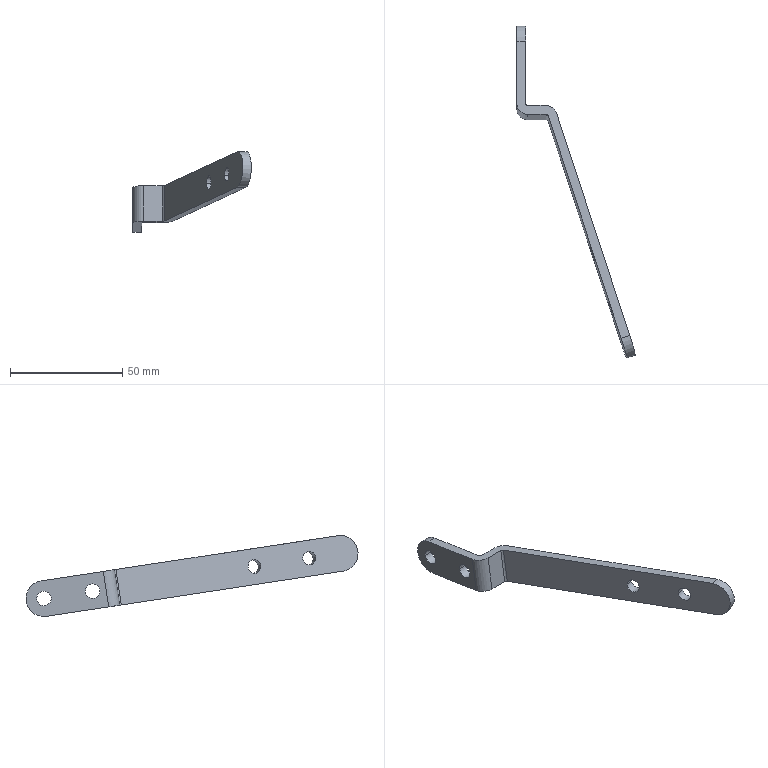Part | SolidWorks | features BaseBody 1 | 1 solid | 23 faces | box 52.887 x 148.089 x 36.172 mm | volume 9906 mm3 | cylinder 15 | plane 8 | commonest cylinder face diameters 6.1 x4 6.5 x4 16 x3 2 x2 10 x2
STEP:
#1=CARTESIAN_POINT('',(27.037,49.349,-203.779));
#2=VERTEX_POINT('',#1);
#3=CARTESIAN_POINT('',(27.037,42.645,-194.665));
#4=VERTEX_POINT('',#3);
#5=CARTESIAN_POINT('',(27.037,41.44,-202.574));
#6=DIRECTION('',(1.,0.,0.));
#7=DIRECTION('',(0.,0.9886,-0.1506));
#8=AXIS2_PLACEMENT_3D('',#5,#6,#7);
#9=CIRCLE('',#8,8.);
#10=EDGE_CURVE('',#2,#4,#9,.T.);
#11=ORIENTED_EDGE('',*,*,#10,.F.);
#12=CARTESIAN_POINT('',(23.037,49.349,-203.779));
#13=VERTEX_POINT('',#12);
#14=CARTESIAN_POINT('',(23.037,49.349,-203.779));
#15=DIRECTION('',(-1.,0.,0.));
#16=VECTOR('',#15,1000.);
#17=LINE('',#14,#16);
#18=EDGE_CURVE('',#2,#13,#17,.T.);
#19=ORIENTED_EDGE('',*,*,#18,.T.);
#20=CARTESIAN_POINT('',(23.037,42.645,-194.665));
#21=VERTEX_POINT('',#20);
#22=CARTESIAN_POINT('',(23.037,41.44,-202.574));
#23=DIRECTION('',(-1.,0.,0.));
#24=DIRECTION('',(0.,0.9886,-0.1506));
#25=AXIS2_PLACEMENT_3D('',#22,#23,#24);
#26=CIRCLE('',#25,8.);
#27=EDGE_CURVE('',#21,#13,#26,.T.);
#28=ORIENTED_EDGE('',*,*,#27,.F.);
#29=CARTESIAN_POINT('',(23.037,42.645,-194.665));
#30=DIRECTION('',(-1.,0.,0.));
#31=VECTOR('',#30,1000.);
#32=LINE('',#29,#31);
#33=EDGE_CURVE('',#4,#21,#32,.T.);
#34=ORIENTED_EDGE('',*,*,#33,.F.);
#35=EDGE_LOOP('',(#11,#19,#28,#34));
#36=FACE_OUTER_BOUND('',#35,.T.);
#37=CARTESIAN_POINT('',(23.037,41.44,-202.574));
#38=DIRECTION('',(-1.,0.,0.));
#39=DIRECTION('',(0.,0.9886,-0.1506));
#40=AXIS2_PLACEMENT_3D('',#37,#38,#39);
#41=CYLINDRICAL_SURFACE('',#40,8.);
#42=ADVANCED_FACE('',(#36),#41,.T.);
#43=CARTESIAN_POINT('',(23.037,38.227,-202.085));
#44=VERTEX_POINT('',#43);
#45=CARTESIAN_POINT('',(23.037,44.653,-203.064));
#46=VERTEX_POINT('',#45);
#47=CARTESIAN_POINT('',(23.037,41.44,-202.574));
#48=DIRECTION('',(-1.,0.,0.));
#49=DIRECTION('',(0.,0.9886,-0.1506));
#50=AXIS2_PLACEMENT_3D('',#47,#48,#49);
#51=CIRCLE('',#50,3.25);
#52=EDGE_CURVE('',#44,#46,#51,.T.);
#53=ORIENTED_EDGE('',*,*,#52,.T.);
#54=CARTESIAN_POINT('',(27.037,44.653,-203.064));
#55=VERTEX_POINT('',#54);
#56=CARTESIAN_POINT('',(17.037,44.653,-203.064));
#57=DIRECTION('',(1.,0.,0.));
#58=VECTOR('',#57,1000.);
#59=LINE('',#56,#58);
#60=EDGE_CURVE('',#46,#55,#59,.T.);
#61=ORIENTED_EDGE('',*,*,#60,.T.);
#62=CARTESIAN_POINT('',(27.037,38.227,-202.085));
#63=VERTEX_POINT('',#62);
#64=CARTESIAN_POINT('',(27.037,41.44,-202.574));
#65=DIRECTION('',(1.,0.,0.));
#66=DIRECTION('',(0.,-0.9886,0.1506));
#67=AXIS2_PLACEMENT_3D('',#64,#65,#66);
#68=CIRCLE('',#67,3.25);
#69=EDGE_CURVE('',#55,#63,#68,.T.);
#70=ORIENTED_EDGE('',*,*,#69,.T.);
#71=CARTESIAN_POINT('',(17.037,38.227,-202.085));
#72=DIRECTION('',(1.,0.,0.));
#73=VECTOR('',#72,1000.);
#74=LINE('',#71,#73);
#75=EDGE_CURVE('',#44,#63,#74,.T.);
#76=ORIENTED_EDGE('',*,*,#75,.F.);
#77=EDGE_LOOP('',(#53,#61,#70,#76));
#78=FACE_OUTER_BOUND('',#77,.T.);
#79=CARTESIAN_POINT('',(17.037,41.44,-202.574));
#80=DIRECTION('',(1.,0.,0.));
#81=DIRECTION('',(0.,-0.9886,0.1506));
#82=AXIS2_PLACEMENT_3D('',#79,#80,#81);
#83=CYLINDRICAL_SURFACE('',#82,3.25);
#84=ADVANCED_FACE('',(#78),#83,.F.);
#85=CARTESIAN_POINT('',(23.037,16.478,-198.771));
#86=VERTEX_POINT('',#85);
#87=CARTESIAN_POINT('',(23.037,22.904,-199.75));
#88=VERTEX_POINT('',#87);
#89=CARTESIAN_POINT('',(23.037,19.691,-199.261));
#90=DIRECTION('',(-1.,0.,0.));
#91=DIRECTION('',(0.,0.9886,-0.1506));
#92=AXIS2_PLACEMENT_3D('',#89,#90,#91);
#93=CIRCLE('',#92,3.25);
#94=EDGE_CURVE('',#86,#88,#93,.T.);
#95=ORIENTED_EDGE('',*,*,#94,.T.);
#96=CARTESIAN_POINT('',(27.037,22.904,-199.75));
#97=VERTEX_POINT('',#96);
#98=CARTESIAN_POINT('',(17.037,22.904,-199.75));
#99=DIRECTION('',(1.,0.,0.));
#100=VECTOR('',#99,1000.);
#101=LINE('',#98,#100);
#102=EDGE_CURVE('',#88,#97,#101,.T.);
#103=ORIENTED_EDGE('',*,*,#102,.T.);
#104=CARTESIAN_POINT('',(27.037,16.478,-198.771));
#105=VERTEX_POINT('',#104);
#106=CARTESIAN_POINT('',(27.037,19.691,-199.261));
#107=DIRECTION('',(1.,0.,0.));
#108=DIRECTION('',(0.,-0.9886,0.1506));
#109=AXIS2_PLACEMENT_3D('',#106,#107,#108);
#110=CIRCLE('',#109,3.25);
#111=EDGE_CURVE('',#97,#105,#110,.T.);
#112=ORIENTED_EDGE('',*,*,#111,.T.);
#113=CARTESIAN_POINT('',(17.037,16.478,-198.771));
#114=DIRECTION('',(1.,0.,0.));
#115=VECTOR('',#114,1000.);
#116=LINE('',#113,#115);
#117=EDGE_CURVE('',#86,#105,#116,.T.);
#118=ORIENTED_EDGE('',*,*,#117,.F.);
#119=EDGE_LOOP('',(#95,#103,#112,#118));
#120=FACE_OUTER_BOUND('',#119,.T.);
#121=CARTESIAN_POINT('',(17.037,19.691,-199.261));
#122=DIRECTION('',(1.,0.,0.));
#123=DIRECTION('',(0.,-0.9886,0.1506));
#124=AXIS2_PLACEMENT_3D('',#121,#122,#123);
#125=CYLINDRICAL_SURFACE('',#124,3.25);
#126=ADVANCED_FACE('',(#120),#125,.F.);
#127=CARTESIAN_POINT('',(69.759,-78.574,-184.291));
#128=VERTEX_POINT('',#127);
#129=CARTESIAN_POINT('',(67.874,-72.839,-185.165));
#130=VERTEX_POINT('',#129);
#131=CARTESIAN_POINT('',(68.817,-75.707,-184.728));
#132=DIRECTION('',(-0.9511,-0.3055,0.04654));
#133=DIRECTION('',(-0.309,0.9402,-0.1432));
#134=AXIS2_PLACEMENT_3D('',#131,#132,#133);
#135=CIRCLE('',#134,3.05);
#136=EDGE_CURVE('',#128,#130,#135,.T.);
#137=ORIENTED_EDGE('',*,*,#136,.F.);
#138=CARTESIAN_POINT('',(65.955,-79.796,-184.105));
#139=VERTEX_POINT('',#138);
#140=CARTESIAN_POINT('',(65.955,-79.796,-184.105));
#141=DIRECTION('',(-0.9511,-0.3055,0.04654));
#142=VECTOR('',#141,1000.);
#143=LINE('',#140,#142);
#144=EDGE_CURVE('',#128,#139,#143,.T.);
#145=ORIENTED_EDGE('',*,*,#144,.T.);
#146=CARTESIAN_POINT('',(64.07,-74.061,-184.978));
#147=VERTEX_POINT('',#146);
#148=CARTESIAN_POINT('',(65.013,-76.928,-184.542));
#149=DIRECTION('',(-0.9511,-0.3055,0.04654));
#150=DIRECTION('',(-0.309,0.9402,-0.1432));
#151=AXIS2_PLACEMENT_3D('',#148,#149,#150);
#152=CIRCLE('',#151,3.05);
#153=EDGE_CURVE('',#139,#147,#152,.T.);
#154=ORIENTED_EDGE('',*,*,#153,.T.);
#155=CARTESIAN_POINT('',(64.07,-74.061,-184.978));
#156=DIRECTION('',(-0.9511,-0.3055,0.04654));
#157=VECTOR('',#156,1000.);
#158=LINE('',#155,#157);
#159=EDGE_CURVE('',#130,#147,#158,.T.);
#160=ORIENTED_EDGE('',*,*,#159,.F.);
#161=EDGE_LOOP('',(#137,#145,#154,#160));
#162=FACE_OUTER_BOUND('',#161,.T.);
#163=CARTESIAN_POINT('',(65.013,-76.928,-184.542));
#164=DIRECTION('',(-0.9511,-0.3055,0.04654));
#165=DIRECTION('',(-0.309,0.9402,-0.1432));
#166=AXIS2_PLACEMENT_3D('',#163,#164,#165);
#167=CYLINDRICAL_SURFACE('',#166,3.05);
#168=ADVANCED_FACE('',(#162),#167,.F.);
#169=CARTESIAN_POINT('',(61.725,-54.129,-188.015));
#170=VERTEX_POINT('',#169);
#171=CARTESIAN_POINT('',(59.84,-48.393,-188.889));
#172=VERTEX_POINT('',#171);
#173=CARTESIAN_POINT('',(60.782,-51.261,-188.452));
#174=DIRECTION('',(-0.9511,-0.3055,0.04654));
#175=DIRECTION('',(-0.309,0.9402,-0.1432));
#176=AXIS2_PLACEMENT_3D('',#173,#174,#175);
#177=CIRCLE('',#176,3.05);
#178=EDGE_CURVE('',#170,#172,#177,.T.);
#179=ORIENTED_EDGE('',*,*,#178,.F.);
#180=CARTESIAN_POINT('',(57.921,-55.351,-187.829));
#181=VERTEX_POINT('',#180);
#182=CARTESIAN_POINT('',(57.921,-55.351,-187.829));
#183=DIRECTION('',(-0.9511,-0.3055,0.04654));
#184=VECTOR('',#183,1000.);
#185=LINE('',#182,#184);
#186=EDGE_CURVE('',#170,#181,#185,.T.);
#187=ORIENTED_EDGE('',*,*,#186,.T.);
#188=CARTESIAN_POINT('',(56.036,-49.615,-188.703));
#189=VERTEX_POINT('',#188);
#190=CARTESIAN_POINT('',(56.978,-52.483,-188.266));
#191=DIRECTION('',(-0.9511,-0.3055,0.04654));
#192=DIRECTION('',(-0.309,0.9402,-0.1432));
#193=AXIS2_PLACEMENT_3D('',#190,#191,#192);
#194=CIRCLE('',#193,3.05);
#195=EDGE_CURVE('',#181,#189,#194,.T.);
#196=ORIENTED_EDGE('',*,*,#195,.T.);
#197=CARTESIAN_POINT('',(56.036,-49.615,-188.703));
#198=DIRECTION('',(-0.9511,-0.3055,0.04654));
#199=VECTOR('',#198,1000.);
#200=LINE('',#197,#199);
#201=EDGE_CURVE('',#172,#189,#200,.T.);
#202=ORIENTED_EDGE('',*,*,#201,.F.);
#203=EDGE_LOOP('',(#179,#187,#196,#202));
#204=FACE_OUTER_BOUND('',#203,.T.);
#205=CARTESIAN_POINT('',(56.978,-52.483,-188.266));
#206=DIRECTION('',(-0.9511,-0.3055,0.04654));
#207=DIRECTION('',(-0.309,0.9402,-0.1432));
#208=AXIS2_PLACEMENT_3D('',#205,#206,#207);
#209=CYLINDRICAL_SURFACE('',#208,3.05);
#210=ADVANCED_FACE('',(#204),#209,.F.);
#211=CARTESIAN_POINT('',(69.648,-89.827,-174.484));
#212=VERTEX_POINT('',#211);
#213=CARTESIAN_POINT('',(69.648,-92.236,-190.302));
#214=VERTEX_POINT('',#213);
#215=CARTESIAN_POINT('',(69.648,-91.032,-182.393));
#216=DIRECTION('',(0.9511,0.3055,-0.04654));
#217=DIRECTION('',(-0.309,0.9402,-0.1432));
#218=AXIS2_PLACEMENT_3D('',#215,#216,#217);
#219=CIRCLE('',#218,8.);
#220=EDGE_CURVE('',#212,#214,#219,.T.);
#221=ORIENTED_EDGE('',*,*,#220,.T.);
#222=CARTESIAN_POINT('',(73.452,-91.014,-190.488));
#223=VERTEX_POINT('',#222);
#224=CARTESIAN_POINT('',(69.648,-92.236,-190.302));
#225=DIRECTION('',(0.9511,0.3055,-0.04654));
#226=VECTOR('',#225,1000.);
#227=LINE('',#224,#226);
#228=EDGE_CURVE('',#214,#223,#227,.T.);
#229=ORIENTED_EDGE('',*,*,#228,.T.);
#230=CARTESIAN_POINT('',(73.452,-88.605,-174.67));
#231=VERTEX_POINT('',#230);
#232=CARTESIAN_POINT('',(73.452,-89.81,-182.579));
#233=DIRECTION('',(0.9511,0.3055,-0.04654));
#234=DIRECTION('',(-0.309,0.9402,-0.1432));
#235=AXIS2_PLACEMENT_3D('',#232,#233,#234);
#236=CIRCLE('',#235,8.);
#237=EDGE_CURVE('',#231,#223,#236,.T.);
#238=ORIENTED_EDGE('',*,*,#237,.F.);
#239=CARTESIAN_POINT('',(69.648,-89.827,-174.484));
#240=DIRECTION('',(0.9511,0.3055,-0.04654));
#241=VECTOR('',#240,1000.);
#242=LINE('',#239,#241);
#243=EDGE_CURVE('',#212,#231,#242,.T.);
#244=ORIENTED_EDGE('',*,*,#243,.F.);
#245=EDGE_LOOP('',(#221,#229,#238,#244));
#246=FACE_OUTER_BOUND('',#245,.T.);
#247=CARTESIAN_POINT('',(69.648,-91.032,-182.393));
#248=DIRECTION('',(-0.9511,-0.3055,0.04654));
#249=DIRECTION('',(-0.309,0.9402,-0.1432));
#250=AXIS2_PLACEMENT_3D('',#247,#248,#249);
#251=CYLINDRICAL_SURFACE('',#250,8.);
#252=ADVANCED_FACE('',(#246),#251,.T.);
#253=ORIENTED_EDGE('',*,*,#186,.F.);
#254=CARTESIAN_POINT('',(60.782,-51.261,-188.452));
#255=DIRECTION('',(-0.9511,-0.3055,0.04654));
#256=DIRECTION('',(-0.309,0.9402,-0.1432));
#257=AXIS2_PLACEMENT_3D('',#254,#255,#256);
#258=CIRCLE('',#257,3.05);
#259=EDGE_CURVE('',#172,#170,#258,.T.);
#260=ORIENTED_EDGE('',*,*,#259,.F.);
#261=ORIENTED_EDGE('',*,*,#201,.T.);
#262=CARTESIAN_POINT('',(56.978,-52.483,-188.266));
#263=DIRECTION('',(-0.9511,-0.3055,0.04654));
#264=DIRECTION('',(-0.309,0.9402,-0.1432));
#265=AXIS2_PLACEMENT_3D('',#262,#263,#264);
#266=CIRCLE('',#265,3.05);
#267=EDGE_CURVE('',#189,#181,#266,.T.);
#268=ORIENTED_EDGE('',*,*,#267,.T.);
#269=EDGE_LOOP('',(#253,#260,#261,#268));
#270=FACE_OUTER_BOUND('',#269,.T.);
#271=CARTESIAN_POINT('',(56.978,-52.483,-188.266));
#272=DIRECTION('',(-0.9511,-0.3055,0.04654));
#273=DIRECTION('',(-0.309,0.9402,-0.1432));
#274=AXIS2_PLACEMENT_3D('',#271,#272,#273);
#275=CYLINDRICAL_SURFACE('',#274,3.05);
#276=ADVANCED_FACE('',(#270),#275,.F.);
#277=ORIENTED_EDGE('',*,*,#144,.F.);
#278=CARTESIAN_POINT('',(68.817,-75.707,-184.728));
#279=DIRECTION('',(-0.9511,-0.3055,0.04654));
#280=DIRECTION('',(-0.309,0.9402,-0.1432));
#281=AXIS2_PLACEMENT_3D('',#278,#279,#280);
#282=CIRCLE('',#281,3.05);
#283=EDGE_CURVE('',#130,#128,#282,.T.);
#284=ORIENTED_EDGE('',*,*,#283,.F.);
#285=ORIENTED_EDGE('',*,*,#159,.T.);
#286=CARTESIAN_POINT('',(65.013,-76.928,-184.542));
#287=DIRECTION('',(-0.9511,-0.3055,0.04654));
#288=DIRECTION('',(-0.309,0.9402,-0.1432));
#289=AXIS2_PLACEMENT_3D('',#286,#287,#288);
#290=CIRCLE('',#289,3.05);
#291=EDGE_CURVE('',#147,#139,#290,.T.);
#292=ORIENTED_EDGE('',*,*,#291,.T.);
#293=EDGE_LOOP('',(#277,#284,#285,#292));
#294=FACE_OUTER_BOUND('',#293,.T.);
#295=CARTESIAN_POINT('',(65.013,-76.928,-184.542));
#296=DIRECTION('',(-0.9511,-0.3055,0.04654));
#297=DIRECTION('',(-0.309,0.9402,-0.1432));
#298=AXIS2_PLACEMENT_3D('',#295,#296,#297);
#299=CYLINDRICAL_SURFACE('',#298,3.05);
#300=ADVANCED_FACE('',(#294),#299,.F.);
#301=CARTESIAN_POINT('',(40.86,10.56,-189.778));
#302=VERTEX_POINT('',#301);
#303=CARTESIAN_POINT('',(36.104,13.976,-190.298));
#304=VERTEX_POINT('',#303);
#305=CARTESIAN_POINT('',(36.104,9.033,-189.545));
#306=DIRECTION('',(0.,0.1506,0.9886));
#307=DIRECTION('',(1.,0.,0.));
#308=AXIS2_PLACEMENT_3D('',#305,#306,#307);
#309=CIRCLE('',#308,5.);
#310=EDGE_CURVE('',#302,#304,#309,.T.);
#311=ORIENTED_EDGE('',*,*,#310,.F.);
#312=CARTESIAN_POINT('',(40.86,8.15,-205.595));
#313=VERTEX_POINT('',#312);
#314=CARTESIAN_POINT('',(40.86,8.15,-205.595));
#315=DIRECTION('',(0.,0.1506,0.9886));
#316=VECTOR('',#315,1000.);
#317=LINE('',#314,#316);
#318=EDGE_CURVE('',#313,#302,#317,.T.);
#319=ORIENTED_EDGE('',*,*,#318,.F.);
#320=CARTESIAN_POINT('',(36.104,11.566,-206.115));
#321=VERTEX_POINT('',#320);
#322=CARTESIAN_POINT('',(36.104,6.623,-205.362));
#323=DIRECTION('',(0.,-0.1506,-0.9886));
#324=DIRECTION('',(1.,0.,0.));
#325=AXIS2_PLACEMENT_3D('',#322,#323,#324);
#326=CIRCLE('',#325,5.);
#327=EDGE_CURVE('',#321,#313,#326,.T.);
#328=ORIENTED_EDGE('',*,*,#327,.F.);
#329=CARTESIAN_POINT('',(36.104,11.566,-206.115));
#330=DIRECTION('',(0.,0.1506,0.9886));
#331=VECTOR('',#330,1000.);
#332=LINE('',#329,#331);
#333=EDGE_CURVE('',#321,#304,#332,.T.);
#334=ORIENTED_EDGE('',*,*,#333,.T.);
#335=EDGE_LOOP('',(#311,#319,#328,#334));
#336=FACE_OUTER_BOUND('',#335,.T.);
#337=CARTESIAN_POINT('',(36.104,5.28,-214.178));
#338=DIRECTION('',(0.,0.1506,0.9886));
#339=DIRECTION('',(1.,0.,0.));
#340=AXIS2_PLACEMENT_3D('',#337,#338,#339);
#341=CYLINDRICAL_SURFACE('',#340,5.);
#342=ADVANCED_FACE('',(#336),#341,.T.);
#343=CARTESIAN_POINT('',(37.055,9.338,-189.591));
#344=VERTEX_POINT('',#343);
#345=CARTESIAN_POINT('',(36.104,10.021,-189.695));
#346=VERTEX_POINT('',#345);
#347=CARTESIAN_POINT('',(36.104,9.033,-189.545));
#348=DIRECTION('',(0.,0.1506,0.9886));
#349=DIRECTION('',(-1.,0.,0.));
#350=AXIS2_PLACEMENT_3D('',#347,#348,#349);
#351=CIRCLE('',#350,1.);
#352=EDGE_CURVE('',#344,#346,#351,.T.);
#353=ORIENTED_EDGE('',*,*,#352,.T.);
#354=CARTESIAN_POINT('',(36.104,7.612,-205.513));
#355=VERTEX_POINT('',#354);
#356=CARTESIAN_POINT('',(36.104,7.612,-205.513));
#357=DIRECTION('',(0.,0.1506,0.9886));
#358=VECTOR('',#357,1000.);
#359=LINE('',#356,#358);
#360=EDGE_CURVE('',#355,#346,#359,.T.);
#361=ORIENTED_EDGE('',*,*,#360,.F.);
#362=CARTESIAN_POINT('',(37.055,6.928,-205.409));
#363=VERTEX_POINT('',#362);
#364=CARTESIAN_POINT('',(36.104,6.623,-205.362));
#365=DIRECTION('',(0.,-0.1506,-0.9886));
#366=DIRECTION('',(-1.,0.,0.));
#367=AXIS2_PLACEMENT_3D('',#364,#365,#366);
#368=CIRCLE('',#367,1.);
#369=EDGE_CURVE('',#355,#363,#368,.T.);
#370=ORIENTED_EDGE('',*,*,#369,.T.);
#371=CARTESIAN_POINT('',(37.055,6.928,-205.409));
#372=DIRECTION('',(0.,0.1506,0.9886));
#373=VECTOR('',#372,1000.);
#374=LINE('',#371,#373);
#375=EDGE_CURVE('',#363,#344,#374,.T.);
#376=ORIENTED_EDGE('',*,*,#375,.T.);
#377=EDGE_LOOP('',(#353,#361,#370,#376));
#378=FACE_OUTER_BOUND('',#377,.T.);
#379=CARTESIAN_POINT('',(36.104,5.28,-214.178));
#380=DIRECTION('',(0.,0.1506,0.9886));
#381=DIRECTION('',(1.,0.,0.));
#382=AXIS2_PLACEMENT_3D('',#379,#380,#381);
#383=CYLINDRICAL_SURFACE('',#382,1.);
#384=ADVANCED_FACE('',(#378),#383,.F.);
#385=ORIENTED_EDGE('',*,*,#102,.F.);
#386=CARTESIAN_POINT('',(23.037,19.691,-199.261));
#387=DIRECTION('',(-1.,0.,0.));
#388=DIRECTION('',(0.,0.9886,-0.1506));
#389=AXIS2_PLACEMENT_3D('',#386,#387,#388);
#390=CIRCLE('',#389,3.25);
#391=EDGE_CURVE('',#88,#86,#390,.T.);
#392=ORIENTED_EDGE('',*,*,#391,.T.);
#393=ORIENTED_EDGE('',*,*,#117,.T.);
#394=CARTESIAN_POINT('',(27.037,19.691,-199.261));
#395=DIRECTION('',(1.,0.,0.));
#396=DIRECTION('',(0.,-0.9886,0.1506));
#397=AXIS2_PLACEMENT_3D('',#394,#395,#396);
#398=CIRCLE('',#397,3.25);
#399=EDGE_CURVE('',#105,#97,#398,.T.);
#400=ORIENTED_EDGE('',*,*,#399,.T.);
#401=EDGE_LOOP('',(#385,#392,#393,#400));
#402=FACE_OUTER_BOUND('',#401,.T.);
#403=CARTESIAN_POINT('',(17.037,19.691,-199.261));
#404=DIRECTION('',(1.,0.,0.));
#405=DIRECTION('',(0.,-0.9886,0.1506));
#406=AXIS2_PLACEMENT_3D('',#403,#404,#405);
#407=CYLINDRICAL_SURFACE('',#406,3.25);
#408=ADVANCED_FACE('',(#402),#407,.F.);
#409=ORIENTED_EDGE('',*,*,#60,.F.);
#410=CARTESIAN_POINT('',(23.037,41.44,-202.574));
#411=DIRECTION('',(-1.,0.,0.));
#412=DIRECTION('',(0.,0.9886,-0.1506));
#413=AXIS2_PLACEMENT_3D('',#410,#411,#412);
#414=CIRCLE('',#413,3.25);
#415=EDGE_CURVE('',#46,#44,#414,.T.);
#416=ORIENTED_EDGE('',*,*,#415,.T.);
#417=ORIENTED_EDGE('',*,*,#75,.T.);
#418=CARTESIAN_POINT('',(27.037,41.44,-202.574));
#419=DIRECTION('',(1.,0.,0.));
#420=DIRECTION('',(0.,-0.9886,0.1506));
#421=AXIS2_PLACEMENT_3D('',#418,#419,#420);
#422=CIRCLE('',#421,3.25);
#423=EDGE_CURVE('',#63,#55,#422,.T.);
#424=ORIENTED_EDGE('',*,*,#423,.T.);
#425=EDGE_LOOP('',(#409,#416,#417,#424));
#426=FACE_OUTER_BOUND('',#425,.T.);
#427=CARTESIAN_POINT('',(17.037,41.44,-202.574));
#428=DIRECTION('',(1.,0.,0.));
#429=DIRECTION('',(0.,-0.9886,0.1506));
#430=AXIS2_PLACEMENT_3D('',#427,#428,#429);
#431=CYLINDRICAL_SURFACE('',#430,3.25);
#432=ADVANCED_FACE('',(#426),#431,.F.);
#433=CARTESIAN_POINT('',(27.037,14.964,-190.449));
#434=VERTEX_POINT('',#433);
#435=CARTESIAN_POINT('',(27.037,12.555,-206.266));
#436=VERTEX_POINT('',#435);
#437=CARTESIAN_POINT('',(27.037,12.555,-206.266));
#438=DIRECTION('',(0.,-0.1506,-0.9886));
#439=VECTOR('',#438,1000.);
#440=LINE('',#437,#439);
#441=EDGE_CURVE('',#434,#436,#440,.T.);
#442=ORIENTED_EDGE('',*,*,#441,.F.);
#443=CARTESIAN_POINT('',(28.037,13.976,-190.298));
#444=VERTEX_POINT('',#443);
#445=CARTESIAN_POINT('',(28.037,14.964,-190.449));
#446=DIRECTION('',(0.,-0.1506,-0.9886));
#447=DIRECTION('',(1.,0.,0.));
#448=AXIS2_PLACEMENT_3D('',#445,#446,#447);
#449=CIRCLE('',#448,1.);
#450=EDGE_CURVE('',#444,#434,#449,.T.);
#451=ORIENTED_EDGE('',*,*,#450,.F.);
#452=CARTESIAN_POINT('',(28.037,11.566,-206.115));
#453=VERTEX_POINT('',#452);
#454=CARTESIAN_POINT('',(28.037,11.566,-206.115));
#455=DIRECTION('',(0.,-0.1506,-0.9886));
#456=VECTOR('',#455,1000.);
#457=LINE('',#454,#456);
#458=EDGE_CURVE('',#444,#453,#457,.T.);
#459=ORIENTED_EDGE('',*,*,#458,.T.);
#460=CARTESIAN_POINT('',(28.037,12.555,-206.266));
#461=DIRECTION('',(0.,0.1506,0.9886));
#462=DIRECTION('',(1.,0.,0.));
#463=AXIS2_PLACEMENT_3D('',#460,#461,#462);
#464=CIRCLE('',#463,1.);
#465=EDGE_CURVE('',#436,#453,#464,.T.);
#466=ORIENTED_EDGE('',*,*,#465,.F.);
#467=EDGE_LOOP('',(#442,#451,#459,#466));
#468=FACE_OUTER_BOUND('',#467,.T.);
#469=CARTESIAN_POINT('',(28.037,11.176,-215.314));
#470=DIRECTION('',(0.,0.1506,0.9886));
#471=DIRECTION('',(1.,0.,0.));
#472=AXIS2_PLACEMENT_3D('',#469,#470,#471);
#473=CYLINDRICAL_SURFACE('',#472,1.);
#474=ADVANCED_FACE('',(#468),#473,.F.);
#475=CARTESIAN_POINT('',(23.037,14.964,-190.449));
#476=VERTEX_POINT('',#475);
#477=CARTESIAN_POINT('',(23.037,12.555,-206.266));
#478=VERTEX_POINT('',#477);
#479=CARTESIAN_POINT('',(23.037,12.555,-206.266));
#480=DIRECTION('',(0.,-0.1506,-0.9886));
#481=VECTOR('',#480,1000.);
#482=LINE('',#479,#481);
#483=EDGE_CURVE('',#476,#478,#482,.T.);
#484=ORIENTED_EDGE('',*,*,#483,.T.);
#485=CARTESIAN_POINT('',(28.037,7.612,-205.513));
#486=VERTEX_POINT('',#485);
#487=CARTESIAN_POINT('',(28.037,12.555,-206.266));
#488=DIRECTION('',(0.,0.1506,0.9886));
#489=DIRECTION('',(1.,0.,0.));
#490=AXIS2_PLACEMENT_3D('',#487,#488,#489);
#491=CIRCLE('',#490,5.);
#492=EDGE_CURVE('',#478,#486,#491,.T.);
#493=ORIENTED_EDGE('',*,*,#492,.T.);
#494=CARTESIAN_POINT('',(28.037,10.021,-189.695));
#495=VERTEX_POINT('',#494);
#496=CARTESIAN_POINT('',(28.037,7.612,-205.513));
#497=DIRECTION('',(0.,-0.1506,-0.9886));
#498=VECTOR('',#497,1000.);
#499=LINE('',#496,#498);
#500=EDGE_CURVE('',#495,#486,#499,.T.);
#501=ORIENTED_EDGE('',*,*,#500,.F.);
#502=CARTESIAN_POINT('',(28.037,14.964,-190.449));
#503=DIRECTION('',(0.,-0.1506,-0.9886));
#504=DIRECTION('',(1.,0.,0.));
#505=AXIS2_PLACEMENT_3D('',#502,#503,#504);
#506=CIRCLE('',#505,5.);
#507=EDGE_CURVE('',#495,#476,#506,.T.);
#508=ORIENTED_EDGE('',*,*,#507,.T.);
#509=EDGE_LOOP('',(#484,#493,#501,#508));
#510=FACE_OUTER_BOUND('',#509,.T.);
#511=CARTESIAN_POINT('',(28.037,11.176,-215.314));
#512=DIRECTION('',(0.,0.1506,0.9886));
#513=DIRECTION('',(1.,0.,0.));
#514=AXIS2_PLACEMENT_3D('',#511,#512,#513);
#515=CYLINDRICAL_SURFACE('',#514,5.);
#516=ADVANCED_FACE('',(#510),#515,.T.);
#517=CARTESIAN_POINT('',(27.037,40.235,-210.483));
#518=VERTEX_POINT('',#517);
#519=CARTESIAN_POINT('',(27.037,48.144,-211.688));
#520=DIRECTION('',(0.,-0.9886,0.1506));
#521=VECTOR('',#520,1000.);
#522=LINE('',#519,#521);
#523=EDGE_CURVE('',#518,#436,#522,.T.);
#524=ORIENTED_EDGE('',*,*,#523,.F.);
#525=CARTESIAN_POINT('',(27.037,41.44,-202.574));
#526=DIRECTION('',(1.,0.,0.));
#527=DIRECTION('',(0.,0.9886,-0.1506));
#528=AXIS2_PLACEMENT_3D('',#525,#526,#527);
#529=CIRCLE('',#528,8.);
#530=EDGE_CURVE('',#518,#2,#529,.T.);
#531=ORIENTED_EDGE('',*,*,#530,.T.);
#532=ORIENTED_EDGE('',*,*,#10,.T.);
#533=CARTESIAN_POINT('',(27.037,50.554,-195.87));
#534=DIRECTION('',(0.,-0.9886,0.1506));
#535=VECTOR('',#534,1000.);
#536=LINE('',#533,#535);
#537=EDGE_CURVE('',#4,#434,#536,.T.);
#538=ORIENTED_EDGE('',*,*,#537,.T.);
#539=ORIENTED_EDGE('',*,*,#441,.T.);
#540=EDGE_LOOP('',(#524,#531,#532,#538,#539));
#541=FACE_OUTER_BOUND('',#540,.T.);
#542=ORIENTED_EDGE('',*,*,#423,.F.);
#543=ORIENTED_EDGE('',*,*,#69,.F.);
#544=EDGE_LOOP('',(#542,#543));
#545=FACE_BOUND('',#544,.T.);
#546=ORIENTED_EDGE('',*,*,#399,.F.);
#547=ORIENTED_EDGE('',*,*,#111,.F.);
#548=EDGE_LOOP('',(#546,#547));
#549=FACE_BOUND('',#548,.T.);
#550=CARTESIAN_POINT('',(27.037,48.144,-211.688));
#551=DIRECTION('',(-1.,0.,0.));
#552=DIRECTION('',(0.,1.,0.));
#553=AXIS2_PLACEMENT_3D('',#550,#551,#552);
#554=PLANE('',#553);
#555=ADVANCED_FACE('',(#541,#545,#549),#554,.F.);
#556=CARTESIAN_POINT('',(23.037,50.554,-195.87));
#557=DIRECTION('',(0.,-0.9886,0.1506));
#558=VECTOR('',#557,1000.);
#559=LINE('',#556,#558);
#560=EDGE_CURVE('',#21,#476,#559,.T.);
#561=ORIENTED_EDGE('',*,*,#560,.F.);
#562=ORIENTED_EDGE('',*,*,#27,.T.);
#563=CARTESIAN_POINT('',(23.037,40.235,-210.483));
#564=VERTEX_POINT('',#563);
#565=CARTESIAN_POINT('',(23.037,41.44,-202.574));
#566=DIRECTION('',(-1.,0.,0.));
#567=DIRECTION('',(0.,0.9886,-0.1506));
#568=AXIS2_PLACEMENT_3D('',#565,#566,#567);
#569=CIRCLE('',#568,8.);
#570=EDGE_CURVE('',#13,#564,#569,.T.);
#571=ORIENTED_EDGE('',*,*,#570,.T.);
#572=CARTESIAN_POINT('',(23.037,48.144,-211.688));
#573=DIRECTION('',(0.,-0.9886,0.1506));
#574=VECTOR('',#573,1000.);
#575=LINE('',#572,#574);
#576=EDGE_CURVE('',#564,#478,#575,.T.);
#577=ORIENTED_EDGE('',*,*,#576,.T.);
#578=ORIENTED_EDGE('',*,*,#483,.F.);
#579=EDGE_LOOP('',(#561,#562,#571,#577,#578));
#580=FACE_OUTER_BOUND('',#579,.T.);
#581=ORIENTED_EDGE('',*,*,#52,.F.);
#582=ORIENTED_EDGE('',*,*,#415,.F.);
#583=EDGE_LOOP('',(#581,#582));
#584=FACE_BOUND('',#583,.T.);
#585=ORIENTED_EDGE('',*,*,#94,.F.);
#586=ORIENTED_EDGE('',*,*,#391,.F.);
#587=EDGE_LOOP('',(#585,#586));
#588=FACE_BOUND('',#587,.T.);
#589=CARTESIAN_POINT('',(23.037,48.144,-211.688));
#590=DIRECTION('',(-1.,0.,0.));
#591=DIRECTION('',(0.,1.,0.));
#592=AXIS2_PLACEMENT_3D('',#589,#590,#591);
#593=PLANE('',#592);
#594=ADVANCED_FACE('',(#580,#584,#588),#593,.T.);
#595=ORIENTED_EDGE('',*,*,#333,.F.);
#596=CARTESIAN_POINT('',(-12.675,11.566,-206.115));
#597=DIRECTION('',(1.,0.,0.));
#598=VECTOR('',#597,1000.);
#599=LINE('',#596,#598);
#600=EDGE_CURVE('',#453,#321,#599,.T.);
#601=ORIENTED_EDGE('',*,*,#600,.F.);
#602=ORIENTED_EDGE('',*,*,#458,.F.);
#603=CARTESIAN_POINT('',(-12.675,13.976,-190.298));
#604=DIRECTION('',(1.,0.,0.));
#605=VECTOR('',#604,1000.);
#606=LINE('',#603,#605);
#607=EDGE_CURVE('',#444,#304,#606,.T.);
#608=ORIENTED_EDGE('',*,*,#607,.T.);
#609=EDGE_LOOP('',(#595,#601,#602,#608));
#610=FACE_OUTER_BOUND('',#609,.T.);
#611=CARTESIAN_POINT('',(-12.675,11.566,-206.115));
#612=DIRECTION('',(0.,-0.9886,0.1506));
#613=DIRECTION('',(-1.,0.,0.));
#614=AXIS2_PLACEMENT_3D('',#611,#612,#613);
#615=PLANE('',#614);
#616=ADVANCED_FACE('',(#610),#615,.F.);
#617=ORIENTED_EDGE('',*,*,#18,.F.);
#618=ORIENTED_EDGE('',*,*,#530,.F.);
#619=CARTESIAN_POINT('',(27.037,40.235,-210.483));
#620=DIRECTION('',(1.,0.,0.));
#621=VECTOR('',#620,1000.);
#622=LINE('',#619,#621);
#623=EDGE_CURVE('',#564,#518,#622,.T.);
#624=ORIENTED_EDGE('',*,*,#623,.F.);
#625=ORIENTED_EDGE('',*,*,#570,.F.);
#626=EDGE_LOOP('',(#617,#618,#624,#625));
#627=FACE_OUTER_BOUND('',#626,.T.);
#628=CARTESIAN_POINT('',(23.037,41.44,-202.574));
#629=DIRECTION('',(-1.,0.,0.));
#630=DIRECTION('',(0.,0.9886,-0.1506));
#631=AXIS2_PLACEMENT_3D('',#628,#629,#630);
#632=CYLINDRICAL_SURFACE('',#631,8.);
#633=ADVANCED_FACE('',(#627),#632,.T.);
#634=CARTESIAN_POINT('',(-12.675,7.612,-205.513));
#635=DIRECTION('',(1.,0.,0.));
#636=VECTOR('',#635,1000.);
#637=LINE('',#634,#636);
#638=EDGE_CURVE('',#486,#355,#637,.T.);
#639=ORIENTED_EDGE('',*,*,#638,.T.);
#640=ORIENTED_EDGE('',*,*,#360,.T.);
#641=CARTESIAN_POINT('',(-12.675,10.021,-189.695));
#642=DIRECTION('',(1.,0.,0.));
#643=VECTOR('',#642,1000.);
#644=LINE('',#641,#643);
#645=EDGE_CURVE('',#495,#346,#644,.T.);
#646=ORIENTED_EDGE('',*,*,#645,.F.);
#647=ORIENTED_EDGE('',*,*,#500,.T.);
#648=EDGE_LOOP('',(#639,#640,#646,#647));
#649=FACE_OUTER_BOUND('',#648,.T.);
#650=CARTESIAN_POINT('',(-12.675,7.612,-205.513));
#651=DIRECTION('',(0.,-0.9886,0.1506));
#652=DIRECTION('',(-1.,0.,0.));
#653=AXIS2_PLACEMENT_3D('',#650,#651,#652);
#654=PLANE('',#653);
#655=ADVANCED_FACE('',(#649),#654,.T.);
#656=ORIENTED_EDGE('',*,*,#243,.T.);
#657=CARTESIAN_POINT('',(24.621,59.968,-197.304));
#658=DIRECTION('',(0.309,-0.9402,0.1432));
#659=VECTOR('',#658,1000.);
#660=LINE('',#657,#659);
#661=EDGE_CURVE('',#302,#231,#660,.T.);
#662=ORIENTED_EDGE('',*,*,#661,.F.);
#663=ORIENTED_EDGE('',*,*,#310,.T.);
#664=ORIENTED_EDGE('',*,*,#607,.F.);
#665=ORIENTED_EDGE('',*,*,#450,.T.);
#666=ORIENTED_EDGE('',*,*,#537,.F.);
#667=ORIENTED_EDGE('',*,*,#33,.T.);
#668=ORIENTED_EDGE('',*,*,#560,.T.);
#669=ORIENTED_EDGE('',*,*,#507,.F.);
#670=ORIENTED_EDGE('',*,*,#645,.T.);
#671=ORIENTED_EDGE('',*,*,#352,.F.);
#672=CARTESIAN_POINT('',(20.817,58.746,-197.118));
#673=DIRECTION('',(0.309,-0.9402,0.1432));
#674=VECTOR('',#673,1000.);
#675=LINE('',#672,#674);
#676=EDGE_CURVE('',#344,#212,#675,.T.);
#677=ORIENTED_EDGE('',*,*,#676,.T.);
#678=EDGE_LOOP('',(#656,#662,#663,#664,#665,#666,#667,#668,#669,#670,#671,#677));
#679=FACE_OUTER_BOUND('',#678,.T.);
#680=CARTESIAN_POINT('',(24.621,59.968,-197.304));
#681=DIRECTION('',(0.,-0.1506,-0.9886));
#682=DIRECTION('',(0.,-0.9886,0.1506));
#683=AXIS2_PLACEMENT_3D('',#680,#681,#682);
#684=PLANE('',#683);
#685=ADVANCED_FACE('',(#679),#684,.F.);
#686=CARTESIAN_POINT('',(24.621,57.558,-213.122));
#687=DIRECTION('',(0.309,-0.9402,0.1432));
#688=VECTOR('',#687,1000.);
#689=LINE('',#686,#688);
#690=EDGE_CURVE('',#313,#223,#689,.T.);
#691=ORIENTED_EDGE('',*,*,#690,.T.);
#692=ORIENTED_EDGE('',*,*,#228,.F.);
#693=CARTESIAN_POINT('',(20.817,56.336,-212.936));
#694=DIRECTION('',(0.309,-0.9402,0.1432));
#695=VECTOR('',#694,1000.);
#696=LINE('',#693,#695);
#697=EDGE_CURVE('',#363,#214,#696,.T.);
#698=ORIENTED_EDGE('',*,*,#697,.F.);
#699=ORIENTED_EDGE('',*,*,#369,.F.);
#700=ORIENTED_EDGE('',*,*,#638,.F.);
#701=ORIENTED_EDGE('',*,*,#492,.F.);
#702=ORIENTED_EDGE('',*,*,#576,.F.);
#703=ORIENTED_EDGE('',*,*,#623,.T.);
#704=ORIENTED_EDGE('',*,*,#523,.T.);
#705=ORIENTED_EDGE('',*,*,#465,.T.);
#706=ORIENTED_EDGE('',*,*,#600,.T.);
#707=ORIENTED_EDGE('',*,*,#327,.T.);
#708=EDGE_LOOP('',(#691,#692,#698,#699,#700,#701,#702,#703,#704,#705,#706,#707));
#709=FACE_OUTER_BOUND('',#708,.T.);
#710=CARTESIAN_POINT('',(24.621,57.558,-213.122));
#711=DIRECTION('',(0.,-0.1506,-0.9886));
#712=DIRECTION('',(0.,-0.9886,0.1506));
#713=AXIS2_PLACEMENT_3D('',#710,#711,#712);
#714=PLANE('',#713);
#715=ADVANCED_FACE('',(#709),#714,.T.);
#716=ORIENTED_EDGE('',*,*,#237,.T.);
#717=ORIENTED_EDGE('',*,*,#690,.F.);
#718=ORIENTED_EDGE('',*,*,#318,.T.);
#719=ORIENTED_EDGE('',*,*,#661,.T.);
#720=EDGE_LOOP('',(#716,#717,#718,#719));
#721=FACE_OUTER_BOUND('',#720,.T.);
#722=ORIENTED_EDGE('',*,*,#283,.T.);
#723=ORIENTED_EDGE('',*,*,#136,.T.);
#724=EDGE_LOOP('',(#722,#723));
#725=FACE_BOUND('',#724,.T.);
#726=ORIENTED_EDGE('',*,*,#259,.T.);
#727=ORIENTED_EDGE('',*,*,#178,.T.);
#728=EDGE_LOOP('',(#726,#727));
#729=FACE_BOUND('',#728,.T.);
#730=CARTESIAN_POINT('',(24.621,57.558,-213.122));
#731=DIRECTION('',(-0.9511,-0.3055,0.04654));
#732=DIRECTION('',(-0.3058,0.9521,0.));
#733=AXIS2_PLACEMENT_3D('',#730,#731,#732);
#734=PLANE('',#733);
#735=ADVANCED_FACE('',(#721,#725,#729),#734,.F.);
#736=ORIENTED_EDGE('',*,*,#697,.T.);
#737=ORIENTED_EDGE('',*,*,#220,.F.);
#738=ORIENTED_EDGE('',*,*,#676,.F.);
#739=ORIENTED_EDGE('',*,*,#375,.F.);
#740=EDGE_LOOP('',(#736,#737,#738,#739));
#741=FACE_OUTER_BOUND('',#740,.T.);
#742=ORIENTED_EDGE('',*,*,#291,.F.);
#743=ORIENTED_EDGE('',*,*,#153,.F.);
#744=EDGE_LOOP('',(#742,#743));
#745=FACE_BOUND('',#744,.T.);
#746=ORIENTED_EDGE('',*,*,#267,.F.);
#747=ORIENTED_EDGE('',*,*,#195,.F.);
#748=EDGE_LOOP('',(#746,#747));
#749=FACE_BOUND('',#748,.T.);
#750=CARTESIAN_POINT('',(20.817,56.336,-212.936));
#751=DIRECTION('',(-0.9511,-0.3055,0.04654));
#752=DIRECTION('',(-0.3058,0.9521,0.));
#753=AXIS2_PLACEMENT_3D('',#750,#751,#752);
#754=PLANE('',#753);
#755=ADVANCED_FACE('',(#741,#745,#749),#754,.T.);
#756=CLOSED_SHELL('',(#42,#84,#126,#168,#210,#252,#276,#300,#342,#384,#408,#432,#474,#516,#555,#594,#616,#633,#655,#685,#715,#735,#755));
#757=MANIFOLD_SOLID_BREP('',#756);
#758=CARTESIAN_POINT('',(0.,0.,0.));
#759=DIRECTION('',(0.,0.,1.));
#760=DIRECTION('',(1.,0.,0.));
#761=AXIS2_PLACEMENT_3D('',#758,#759,#760);
#762=(LENGTH_UNIT()NAMED_UNIT(*)SI_UNIT(.MILLI.,.METRE.));
#763=UNCERTAINTY_MEASURE_WITH_UNIT(LENGTH_MEASURE(0.00001),#762,'','');
#764=(NAMED_UNIT(*)PLANE_ANGLE_UNIT()SI_UNIT($,.RADIAN.));
#765=(NAMED_UNIT(*)SI_UNIT($,.STERADIAN.)SOLID_ANGLE_UNIT());
#766=(GEOMETRIC_REPRESENTATION_CONTEXT(3)GLOBAL_UNCERTAINTY_ASSIGNED_CONTEXT((#763))GLOBAL_UNIT_ASSIGNED_CONTEXT((#762,#764,#765))REPRESENTATION_CONTEXT('',''));
#767=ADVANCED_BREP_SHAPE_REPRESENTATION('',(#757,#761),#766);